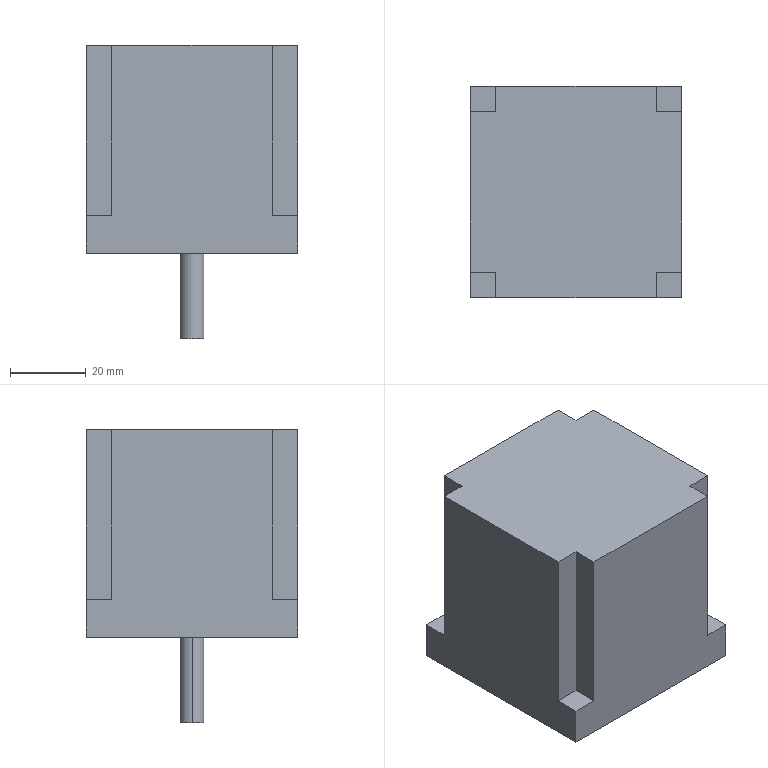Part | STEP file | 57-3260步进马达-2 | 1 solid | 21 faces | box 56 x 56 x 77.6 mm | volume 165142 mm3 | plane 19 | cylinder 2 | commonest cylinder face diameters 6.35 x2
STEP:
#1=CARTESIAN_POINT('',(-3.175,0.,-22.6));
#2=VERTEX_POINT('',#1);
#3=CARTESIAN_POINT('',(3.175,0.,-22.6));
#4=VERTEX_POINT('',#3);
#5=CARTESIAN_POINT('',(0.,0.,-22.6));
#6=DIRECTION('',(0.,0.,-1.));
#7=DIRECTION('',(-1.,0.,0.));
#8=AXIS2_PLACEMENT_3D('',#5,#6,#7);
#9=CIRCLE('',#8,3.175);
#10=EDGE_CURVE('',#2,#4,#9,.T.);
#11=ORIENTED_EDGE('',*,*,#10,.F.);
#12=CARTESIAN_POINT('',(-3.175,0.,0.));
#13=VERTEX_POINT('',#12);
#14=CARTESIAN_POINT('',(-3.175,0.,-22.6));
#15=DIRECTION('',(0.,0.,1.));
#16=VECTOR('',#15,1000.);
#17=LINE('',#14,#16);
#18=EDGE_CURVE('',#2,#13,#17,.T.);
#19=ORIENTED_EDGE('',*,*,#18,.T.);
#20=CARTESIAN_POINT('',(3.175,0.,0.));
#21=VERTEX_POINT('',#20);
#22=CARTESIAN_POINT('',(0.,0.,0.));
#23=DIRECTION('',(0.,0.,-1.));
#24=DIRECTION('',(-1.,0.,0.));
#25=AXIS2_PLACEMENT_3D('',#22,#23,#24);
#26=CIRCLE('',#25,3.175);
#27=EDGE_CURVE('',#13,#21,#26,.T.);
#28=ORIENTED_EDGE('',*,*,#27,.T.);
#29=CARTESIAN_POINT('',(3.175,0.,-22.6));
#30=DIRECTION('',(0.,0.,1.));
#31=VECTOR('',#30,1000.);
#32=LINE('',#29,#31);
#33=EDGE_CURVE('',#4,#21,#32,.T.);
#34=ORIENTED_EDGE('',*,*,#33,.F.);
#35=EDGE_LOOP('',(#11,#19,#28,#34));
#36=FACE_OUTER_BOUND('',#35,.T.);
#37=CARTESIAN_POINT('',(0.,0.,-22.6));
#38=DIRECTION('',(0.,0.,1.));
#39=DIRECTION('',(1.,0.,0.));
#40=AXIS2_PLACEMENT_3D('',#37,#38,#39);
#41=CYLINDRICAL_SURFACE('',#40,3.175);
#42=ADVANCED_FACE('',(#36),#41,.T.);
#43=CARTESIAN_POINT('',(28.,-28.,0.));
#44=VERTEX_POINT('',#43);
#45=CARTESIAN_POINT('',(28.,28.,0.));
#46=VERTEX_POINT('',#45);
#47=CARTESIAN_POINT('',(28.,-28.,0.));
#48=DIRECTION('',(0.,1.,0.));
#49=VECTOR('',#48,1000.);
#50=LINE('',#47,#49);
#51=EDGE_CURVE('',#44,#46,#50,.T.);
#52=ORIENTED_EDGE('',*,*,#51,.F.);
#53=CARTESIAN_POINT('',(-28.,-28.,0.));
#54=VERTEX_POINT('',#53);
#55=CARTESIAN_POINT('',(-28.,-28.,0.));
#56=DIRECTION('',(1.,0.,0.));
#57=VECTOR('',#56,1000.);
#58=LINE('',#55,#57);
#59=EDGE_CURVE('',#54,#44,#58,.T.);
#60=ORIENTED_EDGE('',*,*,#59,.F.);
#61=CARTESIAN_POINT('',(-28.,28.,0.));
#62=VERTEX_POINT('',#61);
#63=CARTESIAN_POINT('',(-28.,-28.,0.));
#64=DIRECTION('',(0.,-1.,0.));
#65=VECTOR('',#64,1000.);
#66=LINE('',#63,#65);
#67=EDGE_CURVE('',#62,#54,#66,.T.);
#68=ORIENTED_EDGE('',*,*,#67,.F.);
#69=CARTESIAN_POINT('',(-28.,28.,0.));
#70=DIRECTION('',(-1.,0.,0.));
#71=VECTOR('',#70,1000.);
#72=LINE('',#69,#71);
#73=EDGE_CURVE('',#46,#62,#72,.T.);
#74=ORIENTED_EDGE('',*,*,#73,.F.);
#75=EDGE_LOOP('',(#52,#60,#68,#74));
#76=FACE_OUTER_BOUND('',#75,.T.);
#77=CARTESIAN_POINT('',(0.,0.,0.));
#78=DIRECTION('',(0.,0.,-1.));
#79=DIRECTION('',(-1.,0.,0.));
#80=AXIS2_PLACEMENT_3D('',#77,#78,#79);
#81=CIRCLE('',#80,3.175);
#82=EDGE_CURVE('',#21,#13,#81,.T.);
#83=ORIENTED_EDGE('',*,*,#82,.F.);
#84=ORIENTED_EDGE('',*,*,#27,.F.);
#85=EDGE_LOOP('',(#83,#84));
#86=FACE_BOUND('',#85,.T.);
#87=CARTESIAN_POINT('',(28.,28.,0.));
#88=DIRECTION('',(0.,0.,-1.));
#89=DIRECTION('',(-1.,0.,0.));
#90=AXIS2_PLACEMENT_3D('',#87,#88,#89);
#91=PLANE('',#90);
#92=ADVANCED_FACE('',(#76,#86),#91,.T.);
#93=CARTESIAN_POINT('',(21.311,21.311,10.));
#94=VERTEX_POINT('',#93);
#95=CARTESIAN_POINT('',(21.311,28.,10.));
#96=VERTEX_POINT('',#95);
#97=CARTESIAN_POINT('',(21.311,28.,10.));
#98=DIRECTION('',(0.,1.,0.));
#99=VECTOR('',#98,1000.);
#100=LINE('',#97,#99);
#101=EDGE_CURVE('',#94,#96,#100,.T.);
#102=ORIENTED_EDGE('',*,*,#101,.F.);
#103=CARTESIAN_POINT('',(28.,21.311,10.));
#104=VERTEX_POINT('',#103);
#105=CARTESIAN_POINT('',(28.,21.311,10.));
#106=DIRECTION('',(-1.,0.,0.));
#107=VECTOR('',#106,1000.);
#108=LINE('',#105,#107);
#109=EDGE_CURVE('',#104,#94,#108,.T.);
#110=ORIENTED_EDGE('',*,*,#109,.F.);
#111=CARTESIAN_POINT('',(28.,28.,10.));
#112=VERTEX_POINT('',#111);
#113=CARTESIAN_POINT('',(28.,-28.,10.));
#114=DIRECTION('',(0.,1.,0.));
#115=VECTOR('',#114,1000.);
#116=LINE('',#113,#115);
#117=EDGE_CURVE('',#104,#112,#116,.T.);
#118=ORIENTED_EDGE('',*,*,#117,.T.);
#119=CARTESIAN_POINT('',(-28.,28.,10.));
#120=DIRECTION('',(-1.,0.,0.));
#121=VECTOR('',#120,1000.);
#122=LINE('',#119,#121);
#123=EDGE_CURVE('',#112,#96,#122,.T.);
#124=ORIENTED_EDGE('',*,*,#123,.T.);
#125=EDGE_LOOP('',(#102,#110,#118,#124));
#126=FACE_OUTER_BOUND('',#125,.T.);
#127=CARTESIAN_POINT('',(28.,28.,10.));
#128=DIRECTION('',(0.,0.,-1.));
#129=DIRECTION('',(-1.,0.,0.));
#130=AXIS2_PLACEMENT_3D('',#127,#128,#129);
#131=PLANE('',#130);
#132=ADVANCED_FACE('',(#126),#131,.F.);
#133=CARTESIAN_POINT('',(21.311,-21.311,10.));
#134=VERTEX_POINT('',#133);
#135=CARTESIAN_POINT('',(28.,-21.311,10.));
#136=VERTEX_POINT('',#135);
#137=CARTESIAN_POINT('',(28.,-21.311,10.));
#138=DIRECTION('',(1.,0.,0.));
#139=VECTOR('',#138,1000.);
#140=LINE('',#137,#139);
#141=EDGE_CURVE('',#134,#136,#140,.T.);
#142=ORIENTED_EDGE('',*,*,#141,.F.);
#143=CARTESIAN_POINT('',(21.311,-28.,10.));
#144=VERTEX_POINT('',#143);
#145=CARTESIAN_POINT('',(21.311,-28.,10.));
#146=DIRECTION('',(0.,1.,0.));
#147=VECTOR('',#146,1000.);
#148=LINE('',#145,#147);
#149=EDGE_CURVE('',#144,#134,#148,.T.);
#150=ORIENTED_EDGE('',*,*,#149,.F.);
#151=CARTESIAN_POINT('',(28.,-28.,10.));
#152=VERTEX_POINT('',#151);
#153=CARTESIAN_POINT('',(-28.,-28.,10.));
#154=DIRECTION('',(1.,0.,0.));
#155=VECTOR('',#154,1000.);
#156=LINE('',#153,#155);
#157=EDGE_CURVE('',#144,#152,#156,.T.);
#158=ORIENTED_EDGE('',*,*,#157,.T.);
#159=CARTESIAN_POINT('',(28.,-28.,10.));
#160=DIRECTION('',(0.,1.,0.));
#161=VECTOR('',#160,1000.);
#162=LINE('',#159,#161);
#163=EDGE_CURVE('',#152,#136,#162,.T.);
#164=ORIENTED_EDGE('',*,*,#163,.T.);
#165=EDGE_LOOP('',(#142,#150,#158,#164));
#166=FACE_OUTER_BOUND('',#165,.T.);
#167=CARTESIAN_POINT('',(28.,28.,10.));
#168=DIRECTION('',(0.,0.,-1.));
#169=DIRECTION('',(-1.,0.,0.));
#170=AXIS2_PLACEMENT_3D('',#167,#168,#169);
#171=PLANE('',#170);
#172=ADVANCED_FACE('',(#166),#171,.F.);
#173=CARTESIAN_POINT('',(-21.311,-21.311,10.));
#174=VERTEX_POINT('',#173);
#175=CARTESIAN_POINT('',(-21.311,-28.,10.));
#176=VERTEX_POINT('',#175);
#177=CARTESIAN_POINT('',(-21.311,-28.,10.));
#178=DIRECTION('',(0.,-1.,0.));
#179=VECTOR('',#178,1000.);
#180=LINE('',#177,#179);
#181=EDGE_CURVE('',#174,#176,#180,.T.);
#182=ORIENTED_EDGE('',*,*,#181,.F.);
#183=CARTESIAN_POINT('',(-28.,-21.311,10.));
#184=VERTEX_POINT('',#183);
#185=CARTESIAN_POINT('',(-28.,-21.311,10.));
#186=DIRECTION('',(1.,0.,0.));
#187=VECTOR('',#186,1000.);
#188=LINE('',#185,#187);
#189=EDGE_CURVE('',#184,#174,#188,.T.);
#190=ORIENTED_EDGE('',*,*,#189,.F.);
#191=CARTESIAN_POINT('',(-28.,-28.,10.));
#192=VERTEX_POINT('',#191);
#193=CARTESIAN_POINT('',(-28.,-28.,10.));
#194=DIRECTION('',(0.,-1.,0.));
#195=VECTOR('',#194,1000.);
#196=LINE('',#193,#195);
#197=EDGE_CURVE('',#184,#192,#196,.T.);
#198=ORIENTED_EDGE('',*,*,#197,.T.);
#199=CARTESIAN_POINT('',(-28.,-28.,10.));
#200=DIRECTION('',(1.,0.,0.));
#201=VECTOR('',#200,1000.);
#202=LINE('',#199,#201);
#203=EDGE_CURVE('',#192,#176,#202,.T.);
#204=ORIENTED_EDGE('',*,*,#203,.T.);
#205=EDGE_LOOP('',(#182,#190,#198,#204));
#206=FACE_OUTER_BOUND('',#205,.T.);
#207=CARTESIAN_POINT('',(28.,28.,10.));
#208=DIRECTION('',(0.,0.,-1.));
#209=DIRECTION('',(-1.,0.,0.));
#210=AXIS2_PLACEMENT_3D('',#207,#208,#209);
#211=PLANE('',#210);
#212=ADVANCED_FACE('',(#206),#211,.F.);
#213=CARTESIAN_POINT('',(-21.311,28.,10.));
#214=VERTEX_POINT('',#213);
#215=CARTESIAN_POINT('',(-21.311,21.311,10.));
#216=VERTEX_POINT('',#215);
#217=CARTESIAN_POINT('',(-21.311,28.,10.));
#218=DIRECTION('',(0.,-1.,0.));
#219=VECTOR('',#218,1000.);
#220=LINE('',#217,#219);
#221=EDGE_CURVE('',#214,#216,#220,.T.);
#222=ORIENTED_EDGE('',*,*,#221,.F.);
#223=CARTESIAN_POINT('',(-28.,28.,10.));
#224=VERTEX_POINT('',#223);
#225=CARTESIAN_POINT('',(-28.,28.,10.));
#226=DIRECTION('',(-1.,0.,0.));
#227=VECTOR('',#226,1000.);
#228=LINE('',#225,#227);
#229=EDGE_CURVE('',#214,#224,#228,.T.);
#230=ORIENTED_EDGE('',*,*,#229,.T.);
#231=CARTESIAN_POINT('',(-28.,21.311,10.));
#232=VERTEX_POINT('',#231);
#233=CARTESIAN_POINT('',(-28.,-28.,10.));
#234=DIRECTION('',(0.,-1.,0.));
#235=VECTOR('',#234,1000.);
#236=LINE('',#233,#235);
#237=EDGE_CURVE('',#224,#232,#236,.T.);
#238=ORIENTED_EDGE('',*,*,#237,.T.);
#239=CARTESIAN_POINT('',(-28.,21.311,10.));
#240=DIRECTION('',(-1.,0.,0.));
#241=VECTOR('',#240,1000.);
#242=LINE('',#239,#241);
#243=EDGE_CURVE('',#216,#232,#242,.T.);
#244=ORIENTED_EDGE('',*,*,#243,.F.);
#245=EDGE_LOOP('',(#222,#230,#238,#244));
#246=FACE_OUTER_BOUND('',#245,.T.);
#247=CARTESIAN_POINT('',(28.,28.,10.));
#248=DIRECTION('',(0.,0.,-1.));
#249=DIRECTION('',(-1.,0.,0.));
#250=AXIS2_PLACEMENT_3D('',#247,#248,#249);
#251=PLANE('',#250);
#252=ADVANCED_FACE('',(#246),#251,.F.);
#253=ORIENTED_EDGE('',*,*,#51,.T.);
#254=CARTESIAN_POINT('',(28.,28.,10.));
#255=DIRECTION('',(0.,0.,-1.));
#256=VECTOR('',#255,1000.);
#257=LINE('',#254,#256);
#258=EDGE_CURVE('',#112,#46,#257,.T.);
#259=ORIENTED_EDGE('',*,*,#258,.F.);
#260=ORIENTED_EDGE('',*,*,#117,.F.);
#261=CARTESIAN_POINT('',(28.,21.311,55.));
#262=VERTEX_POINT('',#261);
#263=CARTESIAN_POINT('',(28.,21.311,55.));
#264=DIRECTION('',(0.,0.,-1.));
#265=VECTOR('',#264,1000.);
#266=LINE('',#263,#265);
#267=EDGE_CURVE('',#262,#104,#266,.T.);
#268=ORIENTED_EDGE('',*,*,#267,.F.);
#269=CARTESIAN_POINT('',(28.,-21.311,55.));
#270=VERTEX_POINT('',#269);
#271=CARTESIAN_POINT('',(28.,-21.311,55.));
#272=DIRECTION('',(0.,1.,0.));
#273=VECTOR('',#272,1000.);
#274=LINE('',#271,#273);
#275=EDGE_CURVE('',#270,#262,#274,.T.);
#276=ORIENTED_EDGE('',*,*,#275,.F.);
#277=CARTESIAN_POINT('',(28.,-21.311,55.));
#278=DIRECTION('',(0.,0.,-1.));
#279=VECTOR('',#278,1000.);
#280=LINE('',#277,#279);
#281=EDGE_CURVE('',#270,#136,#280,.T.);
#282=ORIENTED_EDGE('',*,*,#281,.T.);
#283=ORIENTED_EDGE('',*,*,#163,.F.);
#284=CARTESIAN_POINT('',(28.,-28.,10.));
#285=DIRECTION('',(0.,0.,-1.));
#286=VECTOR('',#285,1000.);
#287=LINE('',#284,#286);
#288=EDGE_CURVE('',#152,#44,#287,.T.);
#289=ORIENTED_EDGE('',*,*,#288,.T.);
#290=EDGE_LOOP('',(#253,#259,#260,#268,#276,#282,#283,#289));
#291=FACE_OUTER_BOUND('',#290,.T.);
#292=CARTESIAN_POINT('',(28.,-28.,10.));
#293=DIRECTION('',(-1.,0.,0.));
#294=DIRECTION('',(0.,0.,1.));
#295=AXIS2_PLACEMENT_3D('',#292,#293,#294);
#296=PLANE('',#295);
#297=ADVANCED_FACE('',(#291),#296,.F.);
#298=ORIENTED_EDGE('',*,*,#73,.T.);
#299=CARTESIAN_POINT('',(-28.,28.,10.));
#300=DIRECTION('',(0.,0.,-1.));
#301=VECTOR('',#300,1000.);
#302=LINE('',#299,#301);
#303=EDGE_CURVE('',#224,#62,#302,.T.);
#304=ORIENTED_EDGE('',*,*,#303,.F.);
#305=ORIENTED_EDGE('',*,*,#229,.F.);
#306=CARTESIAN_POINT('',(-21.311,28.,55.));
#307=VERTEX_POINT('',#306);
#308=CARTESIAN_POINT('',(-21.311,28.,55.));
#309=DIRECTION('',(0.,0.,-1.));
#310=VECTOR('',#309,1000.);
#311=LINE('',#308,#310);
#312=EDGE_CURVE('',#307,#214,#311,.T.);
#313=ORIENTED_EDGE('',*,*,#312,.F.);
#314=CARTESIAN_POINT('',(21.311,28.,55.));
#315=VERTEX_POINT('',#314);
#316=CARTESIAN_POINT('',(-21.311,28.,55.));
#317=DIRECTION('',(-1.,0.,0.));
#318=VECTOR('',#317,1000.);
#319=LINE('',#316,#318);
#320=EDGE_CURVE('',#315,#307,#319,.T.);
#321=ORIENTED_EDGE('',*,*,#320,.F.);
#322=CARTESIAN_POINT('',(21.311,28.,55.));
#323=DIRECTION('',(0.,0.,-1.));
#324=VECTOR('',#323,1000.);
#325=LINE('',#322,#324);
#326=EDGE_CURVE('',#315,#96,#325,.T.);
#327=ORIENTED_EDGE('',*,*,#326,.T.);
#328=ORIENTED_EDGE('',*,*,#123,.F.);
#329=ORIENTED_EDGE('',*,*,#258,.T.);
#330=EDGE_LOOP('',(#298,#304,#305,#313,#321,#327,#328,#329));
#331=FACE_OUTER_BOUND('',#330,.T.);
#332=CARTESIAN_POINT('',(-28.,28.,10.));
#333=DIRECTION('',(0.,-1.,0.));
#334=DIRECTION('',(0.,0.,-1.));
#335=AXIS2_PLACEMENT_3D('',#332,#333,#334);
#336=PLANE('',#335);
#337=ADVANCED_FACE('',(#331),#336,.F.);
#338=ORIENTED_EDGE('',*,*,#67,.T.);
#339=CARTESIAN_POINT('',(-28.,-28.,10.));
#340=DIRECTION('',(0.,0.,-1.));
#341=VECTOR('',#340,1000.);
#342=LINE('',#339,#341);
#343=EDGE_CURVE('',#192,#54,#342,.T.);
#344=ORIENTED_EDGE('',*,*,#343,.F.);
#345=ORIENTED_EDGE('',*,*,#197,.F.);
#346=CARTESIAN_POINT('',(-28.,-21.311,55.));
#347=VERTEX_POINT('',#346);
#348=CARTESIAN_POINT('',(-28.,-21.311,55.));
#349=DIRECTION('',(0.,0.,-1.));
#350=VECTOR('',#349,1000.);
#351=LINE('',#348,#350);
#352=EDGE_CURVE('',#347,#184,#351,.T.);
#353=ORIENTED_EDGE('',*,*,#352,.F.);
#354=CARTESIAN_POINT('',(-28.,21.311,55.));
#355=VERTEX_POINT('',#354);
#356=CARTESIAN_POINT('',(-28.,-21.311,55.));
#357=DIRECTION('',(0.,-1.,0.));
#358=VECTOR('',#357,1000.);
#359=LINE('',#356,#358);
#360=EDGE_CURVE('',#355,#347,#359,.T.);
#361=ORIENTED_EDGE('',*,*,#360,.F.);
#362=CARTESIAN_POINT('',(-28.,21.311,55.));
#363=DIRECTION('',(0.,0.,-1.));
#364=VECTOR('',#363,1000.);
#365=LINE('',#362,#364);
#366=EDGE_CURVE('',#355,#232,#365,.T.);
#367=ORIENTED_EDGE('',*,*,#366,.T.);
#368=ORIENTED_EDGE('',*,*,#237,.F.);
#369=ORIENTED_EDGE('',*,*,#303,.T.);
#370=EDGE_LOOP('',(#338,#344,#345,#353,#361,#367,#368,#369));
#371=FACE_OUTER_BOUND('',#370,.T.);
#372=CARTESIAN_POINT('',(-28.,-28.,10.));
#373=DIRECTION('',(1.,0.,0.));
#374=DIRECTION('',(0.,0.,-1.));
#375=AXIS2_PLACEMENT_3D('',#372,#373,#374);
#376=PLANE('',#375);
#377=ADVANCED_FACE('',(#371),#376,.F.);
#378=ORIENTED_EDGE('',*,*,#59,.T.);
#379=ORIENTED_EDGE('',*,*,#288,.F.);
#380=ORIENTED_EDGE('',*,*,#157,.F.);
#381=CARTESIAN_POINT('',(21.311,-28.,55.));
#382=VERTEX_POINT('',#381);
#383=CARTESIAN_POINT('',(21.311,-28.,55.));
#384=DIRECTION('',(0.,0.,-1.));
#385=VECTOR('',#384,1000.);
#386=LINE('',#383,#385);
#387=EDGE_CURVE('',#382,#144,#386,.T.);
#388=ORIENTED_EDGE('',*,*,#387,.F.);
#389=CARTESIAN_POINT('',(-21.311,-28.,55.));
#390=VERTEX_POINT('',#389);
#391=CARTESIAN_POINT('',(-21.311,-28.,55.));
#392=DIRECTION('',(1.,0.,0.));
#393=VECTOR('',#392,1000.);
#394=LINE('',#391,#393);
#395=EDGE_CURVE('',#390,#382,#394,.T.);
#396=ORIENTED_EDGE('',*,*,#395,.F.);
#397=CARTESIAN_POINT('',(-21.311,-28.,55.));
#398=DIRECTION('',(0.,0.,-1.));
#399=VECTOR('',#398,1000.);
#400=LINE('',#397,#399);
#401=EDGE_CURVE('',#390,#176,#400,.T.);
#402=ORIENTED_EDGE('',*,*,#401,.T.);
#403=ORIENTED_EDGE('',*,*,#203,.F.);
#404=ORIENTED_EDGE('',*,*,#343,.T.);
#405=EDGE_LOOP('',(#378,#379,#380,#388,#396,#402,#403,#404));
#406=FACE_OUTER_BOUND('',#405,.T.);
#407=CARTESIAN_POINT('',(-28.,-28.,10.));
#408=DIRECTION('',(0.,1.,0.));
#409=DIRECTION('',(0.,0.,1.));
#410=AXIS2_PLACEMENT_3D('',#407,#408,#409);
#411=PLANE('',#410);
#412=ADVANCED_FACE('',(#406),#411,.F.);
#413=ORIENTED_EDGE('',*,*,#221,.T.);
#414=CARTESIAN_POINT('',(-21.311,21.311,55.));
#415=VERTEX_POINT('',#414);
#416=CARTESIAN_POINT('',(-21.311,21.311,55.));
#417=DIRECTION('',(0.,0.,-1.));
#418=VECTOR('',#417,1000.);
#419=LINE('',#416,#418);
#420=EDGE_CURVE('',#415,#216,#419,.T.);
#421=ORIENTED_EDGE('',*,*,#420,.F.);
#422=CARTESIAN_POINT('',(-21.311,28.,55.));
#423=DIRECTION('',(0.,-1.,0.));
#424=VECTOR('',#423,1000.);
#425=LINE('',#422,#424);
#426=EDGE_CURVE('',#307,#415,#425,.T.);
#427=ORIENTED_EDGE('',*,*,#426,.F.);
#428=ORIENTED_EDGE('',*,*,#312,.T.);
#429=EDGE_LOOP('',(#413,#421,#427,#428));
#430=FACE_OUTER_BOUND('',#429,.T.);
#431=CARTESIAN_POINT('',(-21.311,28.,55.));
#432=DIRECTION('',(1.,0.,0.));
#433=DIRECTION('',(0.,0.,-1.));
#434=AXIS2_PLACEMENT_3D('',#431,#432,#433);
#435=PLANE('',#434);
#436=ADVANCED_FACE('',(#430),#435,.F.);
#437=ORIENTED_EDGE('',*,*,#243,.T.);
#438=ORIENTED_EDGE('',*,*,#366,.F.);
#439=CARTESIAN_POINT('',(-28.,21.311,55.));
#440=DIRECTION('',(-1.,0.,0.));
#441=VECTOR('',#440,1000.);
#442=LINE('',#439,#441);
#443=EDGE_CURVE('',#415,#355,#442,.T.);
#444=ORIENTED_EDGE('',*,*,#443,.F.);
#445=ORIENTED_EDGE('',*,*,#420,.T.);
#446=EDGE_LOOP('',(#437,#438,#444,#445));
#447=FACE_OUTER_BOUND('',#446,.T.);
#448=CARTESIAN_POINT('',(-28.,21.311,55.));
#449=DIRECTION('',(0.,-1.,0.));
#450=DIRECTION('',(1.,0.,0.));
#451=AXIS2_PLACEMENT_3D('',#448,#449,#450);
#452=PLANE('',#451);
#453=ADVANCED_FACE('',(#447),#452,.F.);
#454=ORIENTED_EDGE('',*,*,#189,.T.);
#455=CARTESIAN_POINT('',(-21.311,-21.311,55.));
#456=VERTEX_POINT('',#455);
#457=CARTESIAN_POINT('',(-21.311,-21.311,55.));
#458=DIRECTION('',(0.,0.,-1.));
#459=VECTOR('',#458,1000.);
#460=LINE('',#457,#459);
#461=EDGE_CURVE('',#456,#174,#460,.T.);
#462=ORIENTED_EDGE('',*,*,#461,.F.);
#463=CARTESIAN_POINT('',(-28.,-21.311,55.));
#464=DIRECTION('',(1.,0.,0.));
#465=VECTOR('',#464,1000.);
#466=LINE('',#463,#465);
#467=EDGE_CURVE('',#347,#456,#466,.T.);
#468=ORIENTED_EDGE('',*,*,#467,.F.);
#469=ORIENTED_EDGE('',*,*,#352,.T.);
#470=EDGE_LOOP('',(#454,#462,#468,#469));
#471=FACE_OUTER_BOUND('',#470,.T.);
#472=CARTESIAN_POINT('',(-28.,-21.311,55.));
#473=DIRECTION('',(0.,1.,0.));
#474=DIRECTION('',(0.,0.,1.));
#475=AXIS2_PLACEMENT_3D('',#472,#473,#474);
#476=PLANE('',#475);
#477=ADVANCED_FACE('',(#471),#476,.F.);
#478=ORIENTED_EDGE('',*,*,#181,.T.);
#479=ORIENTED_EDGE('',*,*,#401,.F.);
#480=CARTESIAN_POINT('',(-21.311,-28.,55.));
#481=DIRECTION('',(0.,-1.,0.));
#482=VECTOR('',#481,1000.);
#483=LINE('',#480,#482);
#484=EDGE_CURVE('',#456,#390,#483,.T.);
#485=ORIENTED_EDGE('',*,*,#484,.F.);
#486=ORIENTED_EDGE('',*,*,#461,.T.);
#487=EDGE_LOOP('',(#478,#479,#485,#486));
#488=FACE_OUTER_BOUND('',#487,.T.);
#489=CARTESIAN_POINT('',(-21.311,-28.,55.));
#490=DIRECTION('',(1.,0.,0.));
#491=DIRECTION('',(0.,0.,-1.));
#492=AXIS2_PLACEMENT_3D('',#489,#490,#491);
#493=PLANE('',#492);
#494=ADVANCED_FACE('',(#488),#493,.F.);
#495=ORIENTED_EDGE('',*,*,#149,.T.);
#496=CARTESIAN_POINT('',(21.311,-21.311,55.));
#497=VERTEX_POINT('',#496);
#498=CARTESIAN_POINT('',(21.311,-21.311,55.));
#499=DIRECTION('',(0.,0.,-1.));
#500=VECTOR('',#499,1000.);
#501=LINE('',#498,#500);
#502=EDGE_CURVE('',#497,#134,#501,.T.);
#503=ORIENTED_EDGE('',*,*,#502,.F.);
#504=CARTESIAN_POINT('',(21.311,-28.,55.));
#505=DIRECTION('',(0.,1.,0.));
#506=VECTOR('',#505,1000.);
#507=LINE('',#504,#506);
#508=EDGE_CURVE('',#382,#497,#507,.T.);
#509=ORIENTED_EDGE('',*,*,#508,.F.);
#510=ORIENTED_EDGE('',*,*,#387,.T.);
#511=EDGE_LOOP('',(#495,#503,#509,#510));
#512=FACE_OUTER_BOUND('',#511,.T.);
#513=CARTESIAN_POINT('',(21.311,-28.,55.));
#514=DIRECTION('',(-1.,0.,0.));
#515=DIRECTION('',(0.,0.,1.));
#516=AXIS2_PLACEMENT_3D('',#513,#514,#515);
#517=PLANE('',#516);
#518=ADVANCED_FACE('',(#512),#517,.F.);
#519=ORIENTED_EDGE('',*,*,#141,.T.);
#520=ORIENTED_EDGE('',*,*,#281,.F.);
#521=CARTESIAN_POINT('',(28.,-21.311,55.));
#522=DIRECTION('',(1.,0.,0.));
#523=VECTOR('',#522,1000.);
#524=LINE('',#521,#523);
#525=EDGE_CURVE('',#497,#270,#524,.T.);
#526=ORIENTED_EDGE('',*,*,#525,.F.);
#527=ORIENTED_EDGE('',*,*,#502,.T.);
#528=EDGE_LOOP('',(#519,#520,#526,#527));
#529=FACE_OUTER_BOUND('',#528,.T.);
#530=CARTESIAN_POINT('',(28.,-21.311,55.));
#531=DIRECTION('',(0.,1.,0.));
#532=DIRECTION('',(0.,0.,1.));
#533=AXIS2_PLACEMENT_3D('',#530,#531,#532);
#534=PLANE('',#533);
#535=ADVANCED_FACE('',(#529),#534,.F.);
#536=ORIENTED_EDGE('',*,*,#109,.T.);
#537=CARTESIAN_POINT('',(21.311,21.311,55.));
#538=VERTEX_POINT('',#537);
#539=CARTESIAN_POINT('',(21.311,21.311,55.));
#540=DIRECTION('',(0.,0.,-1.));
#541=VECTOR('',#540,1000.);
#542=LINE('',#539,#541);
#543=EDGE_CURVE('',#538,#94,#542,.T.);
#544=ORIENTED_EDGE('',*,*,#543,.F.);
#545=CARTESIAN_POINT('',(28.,21.311,55.));
#546=DIRECTION('',(-1.,0.,0.));
#547=VECTOR('',#546,1000.);
#548=LINE('',#545,#547);
#549=EDGE_CURVE('',#262,#538,#548,.T.);
#550=ORIENTED_EDGE('',*,*,#549,.F.);
#551=ORIENTED_EDGE('',*,*,#267,.T.);
#552=EDGE_LOOP('',(#536,#544,#550,#551));
#553=FACE_OUTER_BOUND('',#552,.T.);
#554=CARTESIAN_POINT('',(28.,21.311,55.));
#555=DIRECTION('',(0.,-1.,0.));
#556=DIRECTION('',(0.,0.,-1.));
#557=AXIS2_PLACEMENT_3D('',#554,#555,#556);
#558=PLANE('',#557);
#559=ADVANCED_FACE('',(#553),#558,.F.);
#560=ORIENTED_EDGE('',*,*,#101,.T.);
#561=ORIENTED_EDGE('',*,*,#326,.F.);
#562=CARTESIAN_POINT('',(21.311,28.,55.));
#563=DIRECTION('',(0.,1.,0.));
#564=VECTOR('',#563,1000.);
#565=LINE('',#562,#564);
#566=EDGE_CURVE('',#538,#315,#565,.T.);
#567=ORIENTED_EDGE('',*,*,#566,.F.);
#568=ORIENTED_EDGE('',*,*,#543,.T.);
#569=EDGE_LOOP('',(#560,#561,#567,#568));
#570=FACE_OUTER_BOUND('',#569,.T.);
#571=CARTESIAN_POINT('',(21.311,28.,55.));
#572=DIRECTION('',(-1.,0.,0.));
#573=DIRECTION('',(0.,-1.,0.));
#574=AXIS2_PLACEMENT_3D('',#571,#572,#573);
#575=PLANE('',#574);
#576=ADVANCED_FACE('',(#570),#575,.F.);
#577=ORIENTED_EDGE('',*,*,#426,.T.);
#578=ORIENTED_EDGE('',*,*,#443,.T.);
#579=ORIENTED_EDGE('',*,*,#360,.T.);
#580=ORIENTED_EDGE('',*,*,#467,.T.);
#581=ORIENTED_EDGE('',*,*,#484,.T.);
#582=ORIENTED_EDGE('',*,*,#395,.T.);
#583=ORIENTED_EDGE('',*,*,#508,.T.);
#584=ORIENTED_EDGE('',*,*,#525,.T.);
#585=ORIENTED_EDGE('',*,*,#275,.T.);
#586=ORIENTED_EDGE('',*,*,#549,.T.);
#587=ORIENTED_EDGE('',*,*,#566,.T.);
#588=ORIENTED_EDGE('',*,*,#320,.T.);
#589=EDGE_LOOP('',(#577,#578,#579,#580,#581,#582,#583,#584,#585,#586,#587,#588));
#590=FACE_OUTER_BOUND('',#589,.T.);
#591=CARTESIAN_POINT('',(-21.311,21.311,55.));
#592=DIRECTION('',(0.,0.,1.));
#593=DIRECTION('',(1.,0.,0.));
#594=AXIS2_PLACEMENT_3D('',#591,#592,#593);
#595=PLANE('',#594);
#596=ADVANCED_FACE('',(#590),#595,.T.);
#597=ORIENTED_EDGE('',*,*,#18,.F.);
#598=CARTESIAN_POINT('',(0.,0.,-22.6));
#599=DIRECTION('',(0.,0.,-1.));
#600=DIRECTION('',(-1.,0.,0.));
#601=AXIS2_PLACEMENT_3D('',#598,#599,#600);
#602=CIRCLE('',#601,3.175);
#603=EDGE_CURVE('',#4,#2,#602,.T.);
#604=ORIENTED_EDGE('',*,*,#603,.F.);
#605=ORIENTED_EDGE('',*,*,#33,.T.);
#606=ORIENTED_EDGE('',*,*,#82,.T.);
#607=EDGE_LOOP('',(#597,#604,#605,#606));
#608=FACE_OUTER_BOUND('',#607,.T.);
#609=CARTESIAN_POINT('',(0.,0.,-22.6));
#610=DIRECTION('',(0.,0.,1.));
#611=DIRECTION('',(1.,0.,0.));
#612=AXIS2_PLACEMENT_3D('',#609,#610,#611);
#613=CYLINDRICAL_SURFACE('',#612,3.175);
#614=ADVANCED_FACE('',(#608),#613,.T.);
#615=ORIENTED_EDGE('',*,*,#603,.T.);
#616=ORIENTED_EDGE('',*,*,#10,.T.);
#617=EDGE_LOOP('',(#615,#616));
#618=FACE_OUTER_BOUND('',#617,.T.);
#619=CARTESIAN_POINT('',(0.,0.,-22.6));
#620=DIRECTION('',(0.,0.,-1.));
#621=DIRECTION('',(-1.,0.,0.));
#622=AXIS2_PLACEMENT_3D('',#619,#620,#621);
#623=PLANE('',#622);
#624=ADVANCED_FACE('',(#618),#623,.T.);
#625=CLOSED_SHELL('',(#42,#92,#132,#172,#212,#252,#297,#337,#377,#412,#436,#453,#477,#494,#518,#535,#559,#576,#596,#614,#624));
#626=MANIFOLD_SOLID_BREP('',#625);
#627=CARTESIAN_POINT('',(0.,0.,0.));
#628=DIRECTION('',(0.,0.,1.));
#629=DIRECTION('',(1.,0.,0.));
#630=AXIS2_PLACEMENT_3D('',#627,#628,#629);
#631=(LENGTH_UNIT()NAMED_UNIT(*)SI_UNIT(.MILLI.,.METRE.));
#632=UNCERTAINTY_MEASURE_WITH_UNIT(LENGTH_MEASURE(0.00001),#631,'','');
#633=(NAMED_UNIT(*)PLANE_ANGLE_UNIT()SI_UNIT($,.RADIAN.));
#634=(NAMED_UNIT(*)SI_UNIT($,.STERADIAN.)SOLID_ANGLE_UNIT());
#635=(GEOMETRIC_REPRESENTATION_CONTEXT(3)GLOBAL_UNCERTAINTY_ASSIGNED_CONTEXT((#632))GLOBAL_UNIT_ASSIGNED_CONTEXT((#631,#633,#634))REPRESENTATION_CONTEXT('',''));
#636=ADVANCED_BREP_SHAPE_REPRESENTATION('',(#626,#630),#635);